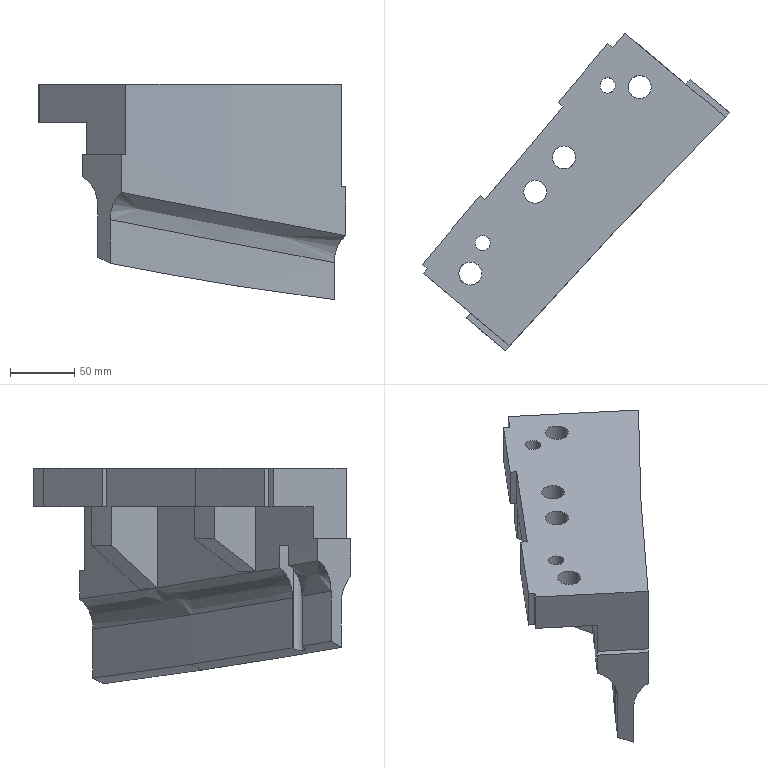Part | NX | features solid 2 | 1 solid | 54 faces | box 239.883 x 248.161 x 168.196 mm | volume 1606272 mm3 | plane 32 | spline 11 | cylinder 11 | commonest cylinder face diameters 18 x4 26 x4 12 x2 10 x1